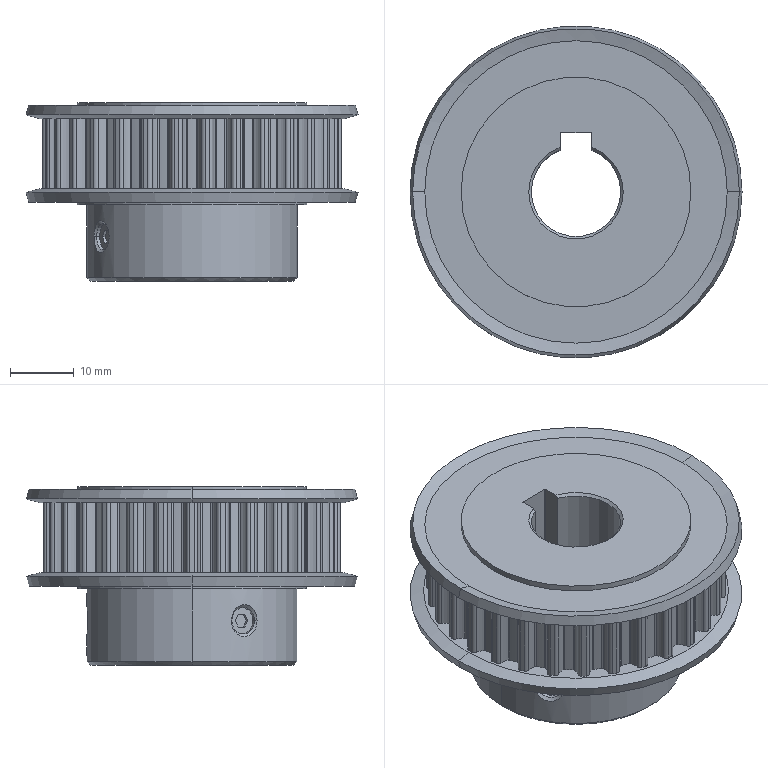Part | SolidWorks | features BaseBody 1 | 1 solid | 305 faces | box 52 x 52 x 28 mm | volume 31408 mm3 | cylinder 257 | plane 28 | cone 20 | commonest cylinder face diameters 0.5 x60 1.1 x60 6.55 x60 43.25 x30 46.79 x30 4.134 x8